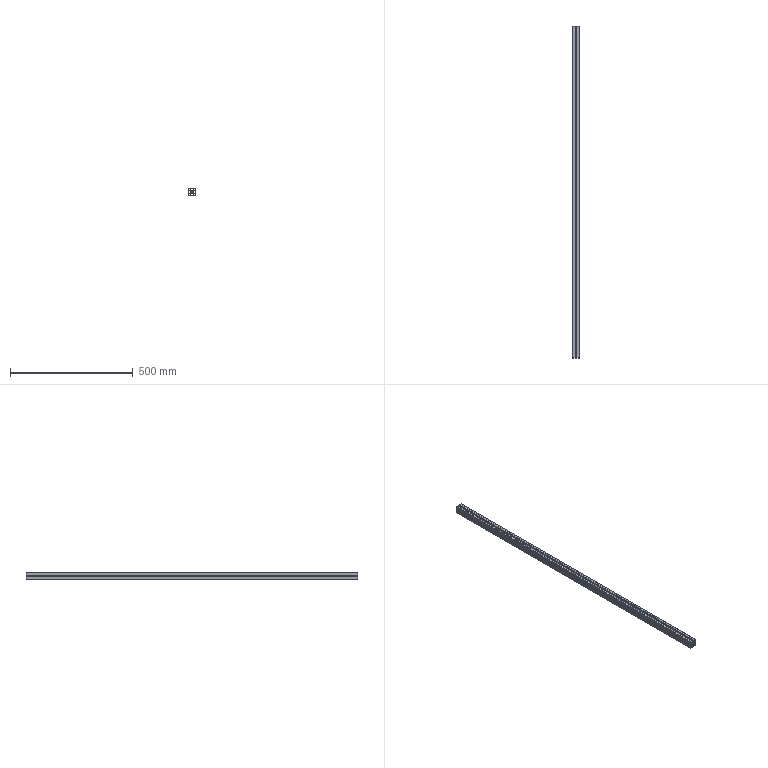Part | STEP file | 08-02 Guard bracket 2 | 1 solid | 137 faces | box 30 x 1350 x 30 mm | volume 569484 mm3 | plane 99 | cylinder 38 | commonest cylinder face diameters 6 x16 6.5 x12 12 x6 2 x4